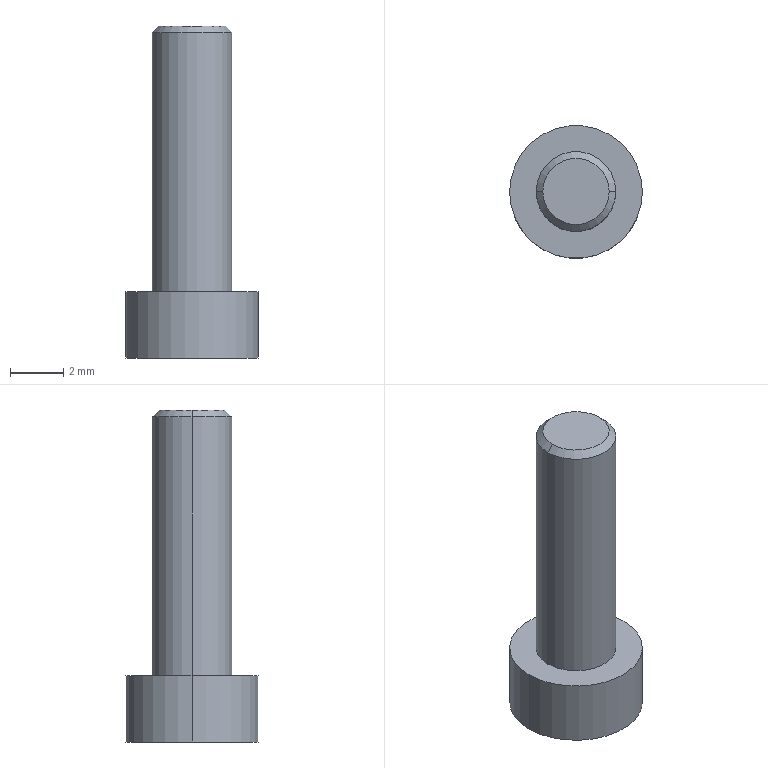Part | SolidWorks | features BaseBody 1 | 1 solid | 16 faces | box 5 x 5 x 12.5 mm | volume 109.752 mm3 | plane 10 | cylinder 4 | cone 2 | commonest cylinder face diameters 3 x2 5 x2
STEP:
#1=CARTESIAN_POINT('',(-1.25,0.,12.5));
#2=VERTEX_POINT('',#1);
#3=CARTESIAN_POINT('',(1.25,0.,12.5));
#4=VERTEX_POINT('',#3);
#5=CARTESIAN_POINT('',(0.,0.,12.5));
#6=DIRECTION('',(0.,0.,-1.));
#7=DIRECTION('',(-1.,0.,0.));
#8=AXIS2_PLACEMENT_3D('',#5,#6,#7);
#9=CIRCLE('',#8,1.25);
#10=EDGE_CURVE('',#2,#4,#9,.T.);
#11=ORIENTED_EDGE('',*,*,#10,.T.);
#12=CARTESIAN_POINT('',(1.5,0.,12.25));
#13=VERTEX_POINT('',#12);
#14=CARTESIAN_POINT('',(1.375,0.,12.375));
#15=DIRECTION('',(0.7071,0.,-0.7071));
#16=VECTOR('',#15,1000.);
#17=LINE('',#14,#16);
#18=EDGE_CURVE('',#4,#13,#17,.T.);
#19=ORIENTED_EDGE('',*,*,#18,.T.);
#20=CARTESIAN_POINT('',(-1.5,0.,12.25));
#21=VERTEX_POINT('',#20);
#22=CARTESIAN_POINT('',(0.,0.,12.25));
#23=DIRECTION('',(0.,0.,1.));
#24=DIRECTION('',(-1.,0.,0.));
#25=AXIS2_PLACEMENT_3D('',#22,#23,#24);
#26=CIRCLE('',#25,1.5);
#27=EDGE_CURVE('',#13,#21,#26,.T.);
#28=ORIENTED_EDGE('',*,*,#27,.T.);
#29=CARTESIAN_POINT('',(-1.375,0.,12.375));
#30=DIRECTION('',(-0.7071,0.,-0.7071));
#31=VECTOR('',#30,1000.);
#32=LINE('',#29,#31);
#33=EDGE_CURVE('',#2,#21,#32,.T.);
#34=ORIENTED_EDGE('',*,*,#33,.F.);
#35=EDGE_LOOP('',(#11,#19,#28,#34));
#36=FACE_OUTER_BOUND('',#35,.T.);
#37=CARTESIAN_POINT('',(0.,0.,12.375));
#38=DIRECTION('',(0.,0.,-1.));
#39=DIRECTION('',(-1.,0.,0.));
#40=AXIS2_PLACEMENT_3D('',#37,#38,#39);
#41=CONICAL_SURFACE('',#40,1.375,0.7854);
#42=ADVANCED_FACE('',(#36),#41,.T.);
#43=ORIENTED_EDGE('',*,*,#27,.F.);
#44=CARTESIAN_POINT('',(1.5,0.,2.5));
#45=VERTEX_POINT('',#44);
#46=CARTESIAN_POINT('',(1.5,0.,2.5));
#47=DIRECTION('',(0.,0.,-1.));
#48=VECTOR('',#47,1000.);
#49=LINE('',#46,#48);
#50=EDGE_CURVE('',#13,#45,#49,.T.);
#51=ORIENTED_EDGE('',*,*,#50,.T.);
#52=CARTESIAN_POINT('',(-1.5,0.,2.5));
#53=VERTEX_POINT('',#52);
#54=CARTESIAN_POINT('',(0.,0.,2.5));
#55=DIRECTION('',(0.,0.,-1.));
#56=DIRECTION('',(-1.,0.,0.));
#57=AXIS2_PLACEMENT_3D('',#54,#55,#56);
#58=CIRCLE('',#57,1.5);
#59=EDGE_CURVE('',#53,#45,#58,.T.);
#60=ORIENTED_EDGE('',*,*,#59,.F.);
#61=CARTESIAN_POINT('',(-1.5,0.,2.5));
#62=DIRECTION('',(0.,0.,-1.));
#63=VECTOR('',#62,1000.);
#64=LINE('',#61,#63);
#65=EDGE_CURVE('',#21,#53,#64,.T.);
#66=ORIENTED_EDGE('',*,*,#65,.F.);
#67=EDGE_LOOP('',(#43,#51,#60,#66));
#68=FACE_OUTER_BOUND('',#67,.T.);
#69=CARTESIAN_POINT('',(0.,0.,2.5));
#70=DIRECTION('',(0.,0.,-1.));
#71=DIRECTION('',(-1.,0.,0.));
#72=AXIS2_PLACEMENT_3D('',#69,#70,#71);
#73=CYLINDRICAL_SURFACE('',#72,1.5);
#74=ADVANCED_FACE('',(#68),#73,.T.);
#75=CARTESIAN_POINT('',(2.5,0.,2.5));
#76=VERTEX_POINT('',#75);
#77=CARTESIAN_POINT('',(-2.5,0.,2.5));
#78=VERTEX_POINT('',#77);
#79=CARTESIAN_POINT('',(0.,0.,2.5));
#80=DIRECTION('',(0.,0.,1.));
#81=DIRECTION('',(-1.,0.,0.));
#82=AXIS2_PLACEMENT_3D('',#79,#80,#81);
#83=CIRCLE('',#82,2.5);
#84=EDGE_CURVE('',#76,#78,#83,.T.);
#85=ORIENTED_EDGE('',*,*,#84,.F.);
#86=CARTESIAN_POINT('',(2.5,0.,0.));
#87=VERTEX_POINT('',#86);
#88=CARTESIAN_POINT('',(2.5,0.,0.));
#89=DIRECTION('',(0.,0.,-1.));
#90=VECTOR('',#89,1000.);
#91=LINE('',#88,#90);
#92=EDGE_CURVE('',#76,#87,#91,.T.);
#93=ORIENTED_EDGE('',*,*,#92,.T.);
#94=CARTESIAN_POINT('',(-2.5,0.,0.));
#95=VERTEX_POINT('',#94);
#96=CARTESIAN_POINT('',(0.,0.,0.));
#97=DIRECTION('',(0.,0.,-1.));
#98=DIRECTION('',(-1.,0.,0.));
#99=AXIS2_PLACEMENT_3D('',#96,#97,#98);
#100=CIRCLE('',#99,2.5);
#101=EDGE_CURVE('',#95,#87,#100,.T.);
#102=ORIENTED_EDGE('',*,*,#101,.F.);
#103=CARTESIAN_POINT('',(-2.5,0.,0.));
#104=DIRECTION('',(0.,0.,-1.));
#105=VECTOR('',#104,1000.);
#106=LINE('',#103,#105);
#107=EDGE_CURVE('',#78,#95,#106,.T.);
#108=ORIENTED_EDGE('',*,*,#107,.F.);
#109=EDGE_LOOP('',(#85,#93,#102,#108));
#110=FACE_OUTER_BOUND('',#109,.T.);
#111=CARTESIAN_POINT('',(0.,0.,0.));
#112=DIRECTION('',(0.,0.,-1.));
#113=DIRECTION('',(-1.,0.,0.));
#114=AXIS2_PLACEMENT_3D('',#111,#112,#113);
#115=CYLINDRICAL_SURFACE('',#114,2.5);
#116=ADVANCED_FACE('',(#110),#115,.T.);
#117=CARTESIAN_POINT('',(-1.732,0.,0.));
#118=VERTEX_POINT('',#117);
#119=CARTESIAN_POINT('',(-0.866,-1.5,0.));
#120=VERTEX_POINT('',#119);
#121=CARTESIAN_POINT('',(-1.516,-0.375,0.));
#122=DIRECTION('',(0.5,-0.866,0.));
#123=VECTOR('',#122,1000.);
#124=LINE('',#121,#123);
#125=EDGE_CURVE('',#118,#120,#124,.T.);
#126=ORIENTED_EDGE('',*,*,#125,.F.);
#127=CARTESIAN_POINT('',(-1.732,0.,1.25));
#128=VERTEX_POINT('',#127);
#129=CARTESIAN_POINT('',(-1.732,0.,0.));
#130=DIRECTION('',(0.,0.,1.));
#131=VECTOR('',#130,1000.);
#132=LINE('',#129,#131);
#133=EDGE_CURVE('',#118,#128,#132,.T.);
#134=ORIENTED_EDGE('',*,*,#133,.T.);
#135=CARTESIAN_POINT('',(-0.866,-1.5,1.25));
#136=VERTEX_POINT('',#135);
#137=CARTESIAN_POINT('',(-1.732,0.,1.25));
#138=DIRECTION('',(0.5,-0.866,0.));
#139=VECTOR('',#138,1000.);
#140=LINE('',#137,#139);
#141=EDGE_CURVE('',#128,#136,#140,.T.);
#142=ORIENTED_EDGE('',*,*,#141,.T.);
#143=CARTESIAN_POINT('',(-0.866,-1.5,0.));
#144=DIRECTION('',(0.,0.,1.));
#145=VECTOR('',#144,1000.);
#146=LINE('',#143,#145);
#147=EDGE_CURVE('',#120,#136,#146,.T.);
#148=ORIENTED_EDGE('',*,*,#147,.F.);
#149=EDGE_LOOP('',(#126,#134,#142,#148));
#150=FACE_OUTER_BOUND('',#149,.T.);
#151=CARTESIAN_POINT('',(-1.732,0.,0.));
#152=DIRECTION('',(-0.866,-0.5,0.));
#153=DIRECTION('',(-0.5,0.866,0.));
#154=AXIS2_PLACEMENT_3D('',#151,#152,#153);
#155=PLANE('',#154);
#156=ADVANCED_FACE('',(#150),#155,.F.);
#157=CARTESIAN_POINT('',(-0.866,1.5,0.));
#158=VERTEX_POINT('',#157);
#159=CARTESIAN_POINT('',(-1.083,1.125,0.));
#160=DIRECTION('',(-0.5,-0.866,0.));
#161=VECTOR('',#160,1000.);
#162=LINE('',#159,#161);
#163=EDGE_CURVE('',#158,#118,#162,.T.);
#164=ORIENTED_EDGE('',*,*,#163,.F.);
#165=CARTESIAN_POINT('',(-0.866,1.5,1.25));
#166=VERTEX_POINT('',#165);
#167=CARTESIAN_POINT('',(-0.866,1.5,0.));
#168=DIRECTION('',(0.,0.,1.));
#169=VECTOR('',#168,1000.);
#170=LINE('',#167,#169);
#171=EDGE_CURVE('',#158,#166,#170,.T.);
#172=ORIENTED_EDGE('',*,*,#171,.T.);
#173=CARTESIAN_POINT('',(-0.866,1.5,1.25));
#174=DIRECTION('',(-0.5,-0.866,0.));
#175=VECTOR('',#174,1000.);
#176=LINE('',#173,#175);
#177=EDGE_CURVE('',#166,#128,#176,.T.);
#178=ORIENTED_EDGE('',*,*,#177,.T.);
#179=ORIENTED_EDGE('',*,*,#133,.F.);
#180=EDGE_LOOP('',(#164,#172,#178,#179));
#181=FACE_OUTER_BOUND('',#180,.T.);
#182=CARTESIAN_POINT('',(-0.866,1.5,0.));
#183=DIRECTION('',(-0.866,0.5,0.));
#184=DIRECTION('',(0.,0.,1.));
#185=AXIS2_PLACEMENT_3D('',#182,#183,#184);
#186=PLANE('',#185);
#187=ADVANCED_FACE('',(#181),#186,.F.);
#188=CARTESIAN_POINT('',(0.866,1.5,0.));
#189=VERTEX_POINT('',#188);
#190=CARTESIAN_POINT('',(0.433,1.5,0.));
#191=DIRECTION('',(-1.,0.,0.));
#192=VECTOR('',#191,1000.);
#193=LINE('',#190,#192);
#194=EDGE_CURVE('',#189,#158,#193,.T.);
#195=ORIENTED_EDGE('',*,*,#194,.F.);
#196=CARTESIAN_POINT('',(0.866,1.5,1.25));
#197=VERTEX_POINT('',#196);
#198=CARTESIAN_POINT('',(0.866,1.5,0.));
#199=DIRECTION('',(0.,0.,1.));
#200=VECTOR('',#199,1000.);
#201=LINE('',#198,#200);
#202=EDGE_CURVE('',#189,#197,#201,.T.);
#203=ORIENTED_EDGE('',*,*,#202,.T.);
#204=CARTESIAN_POINT('',(0.866,1.5,1.25));
#205=DIRECTION('',(-1.,0.,0.));
#206=VECTOR('',#205,1000.);
#207=LINE('',#204,#206);
#208=EDGE_CURVE('',#197,#166,#207,.T.);
#209=ORIENTED_EDGE('',*,*,#208,.T.);
#210=ORIENTED_EDGE('',*,*,#171,.F.);
#211=EDGE_LOOP('',(#195,#203,#209,#210));
#212=FACE_OUTER_BOUND('',#211,.T.);
#213=CARTESIAN_POINT('',(0.866,1.5,0.));
#214=DIRECTION('',(0.,1.,0.));
#215=DIRECTION('',(1.,0.,0.));
#216=AXIS2_PLACEMENT_3D('',#213,#214,#215);
#217=PLANE('',#216);
#218=ADVANCED_FACE('',(#212),#217,.F.);
#219=CARTESIAN_POINT('',(1.732,0.,0.));
#220=VERTEX_POINT('',#219);
#221=CARTESIAN_POINT('',(1.516,0.375,0.));
#222=DIRECTION('',(-0.5,0.866,0.));
#223=VECTOR('',#222,1000.);
#224=LINE('',#221,#223);
#225=EDGE_CURVE('',#220,#189,#224,.T.);
#226=ORIENTED_EDGE('',*,*,#225,.F.);
#227=CARTESIAN_POINT('',(1.732,0.,1.25));
#228=VERTEX_POINT('',#227);
#229=CARTESIAN_POINT('',(1.732,0.,0.));
#230=DIRECTION('',(0.,0.,1.));
#231=VECTOR('',#230,1000.);
#232=LINE('',#229,#231);
#233=EDGE_CURVE('',#220,#228,#232,.T.);
#234=ORIENTED_EDGE('',*,*,#233,.T.);
#235=CARTESIAN_POINT('',(1.732,0.,1.25));
#236=DIRECTION('',(-0.5,0.866,0.));
#237=VECTOR('',#236,1000.);
#238=LINE('',#235,#237);
#239=EDGE_CURVE('',#228,#197,#238,.T.);
#240=ORIENTED_EDGE('',*,*,#239,.T.);
#241=ORIENTED_EDGE('',*,*,#202,.F.);
#242=EDGE_LOOP('',(#226,#234,#240,#241));
#243=FACE_OUTER_BOUND('',#242,.T.);
#244=CARTESIAN_POINT('',(1.732,0.,0.));
#245=DIRECTION('',(0.866,0.5,0.));
#246=DIRECTION('',(0.,0.,-1.));
#247=AXIS2_PLACEMENT_3D('',#244,#245,#246);
#248=PLANE('',#247);
#249=ADVANCED_FACE('',(#243),#248,.F.);
#250=CARTESIAN_POINT('',(0.866,-1.5,0.));
#251=VERTEX_POINT('',#250);
#252=CARTESIAN_POINT('',(1.083,-1.125,0.));
#253=DIRECTION('',(0.5,0.866,0.));
#254=VECTOR('',#253,1000.);
#255=LINE('',#252,#254);
#256=EDGE_CURVE('',#251,#220,#255,.T.);
#257=ORIENTED_EDGE('',*,*,#256,.F.);
#258=CARTESIAN_POINT('',(0.866,-1.5,1.25));
#259=VERTEX_POINT('',#258);
#260=CARTESIAN_POINT('',(0.866,-1.5,0.));
#261=DIRECTION('',(0.,0.,1.));
#262=VECTOR('',#261,1000.);
#263=LINE('',#260,#262);
#264=EDGE_CURVE('',#251,#259,#263,.T.);
#265=ORIENTED_EDGE('',*,*,#264,.T.);
#266=CARTESIAN_POINT('',(0.866,-1.5,1.25));
#267=DIRECTION('',(0.5,0.866,0.));
#268=VECTOR('',#267,1000.);
#269=LINE('',#266,#268);
#270=EDGE_CURVE('',#259,#228,#269,.T.);
#271=ORIENTED_EDGE('',*,*,#270,.T.);
#272=ORIENTED_EDGE('',*,*,#233,.F.);
#273=EDGE_LOOP('',(#257,#265,#271,#272));
#274=FACE_OUTER_BOUND('',#273,.T.);
#275=CARTESIAN_POINT('',(0.866,-1.5,0.));
#276=DIRECTION('',(0.866,-0.5,0.));
#277=DIRECTION('',(0.,0.,-1.));
#278=AXIS2_PLACEMENT_3D('',#275,#276,#277);
#279=PLANE('',#278);
#280=ADVANCED_FACE('',(#274),#279,.F.);
#281=CARTESIAN_POINT('',(-0.433,-1.5,0.));
#282=DIRECTION('',(1.,0.,0.));
#283=VECTOR('',#282,1000.);
#284=LINE('',#281,#283);
#285=EDGE_CURVE('',#120,#251,#284,.T.);
#286=ORIENTED_EDGE('',*,*,#285,.F.);
#287=ORIENTED_EDGE('',*,*,#147,.T.);
#288=CARTESIAN_POINT('',(-0.866,-1.5,1.25));
#289=DIRECTION('',(1.,0.,0.));
#290=VECTOR('',#289,1000.);
#291=LINE('',#288,#290);
#292=EDGE_CURVE('',#136,#259,#291,.T.);
#293=ORIENTED_EDGE('',*,*,#292,.T.);
#294=ORIENTED_EDGE('',*,*,#264,.F.);
#295=EDGE_LOOP('',(#286,#287,#293,#294));
#296=FACE_OUTER_BOUND('',#295,.T.);
#297=CARTESIAN_POINT('',(-0.866,-1.5,0.));
#298=DIRECTION('',(0.,-1.,0.));
#299=DIRECTION('',(0.,0.,-1.));
#300=AXIS2_PLACEMENT_3D('',#297,#298,#299);
#301=PLANE('',#300);
#302=ADVANCED_FACE('',(#296),#301,.F.);
#303=ORIENTED_EDGE('',*,*,#292,.F.);
#304=ORIENTED_EDGE('',*,*,#141,.F.);
#305=ORIENTED_EDGE('',*,*,#177,.F.);
#306=ORIENTED_EDGE('',*,*,#208,.F.);
#307=ORIENTED_EDGE('',*,*,#239,.F.);
#308=ORIENTED_EDGE('',*,*,#270,.F.);
#309=EDGE_LOOP('',(#303,#304,#305,#306,#307,#308));
#310=FACE_OUTER_BOUND('',#309,.T.);
#311=CARTESIAN_POINT('',(0.,0.,1.25));
#312=DIRECTION('',(0.,0.,1.));
#313=DIRECTION('',(1.,0.,0.));
#314=AXIS2_PLACEMENT_3D('',#311,#312,#313);
#315=PLANE('',#314);
#316=ADVANCED_FACE('',(#310),#315,.F.);
#317=ORIENTED_EDGE('',*,*,#10,.F.);
#318=CARTESIAN_POINT('',(0.,0.,12.5));
#319=DIRECTION('',(0.,0.,-1.));
#320=DIRECTION('',(-1.,0.,0.));
#321=AXIS2_PLACEMENT_3D('',#318,#319,#320);
#322=CIRCLE('',#321,1.25);
#323=EDGE_CURVE('',#4,#2,#322,.T.);
#324=ORIENTED_EDGE('',*,*,#323,.F.);
#325=EDGE_LOOP('',(#317,#324));
#326=FACE_OUTER_BOUND('',#325,.T.);
#327=CARTESIAN_POINT('',(0.,0.,12.5));
#328=DIRECTION('',(0.,0.,1.));
#329=DIRECTION('',(1.,0.,0.));
#330=AXIS2_PLACEMENT_3D('',#327,#328,#329);
#331=PLANE('',#330);
#332=ADVANCED_FACE('',(#326),#331,.T.);
#333=ORIENTED_EDGE('',*,*,#125,.T.);
#334=ORIENTED_EDGE('',*,*,#285,.T.);
#335=ORIENTED_EDGE('',*,*,#256,.T.);
#336=ORIENTED_EDGE('',*,*,#225,.T.);
#337=ORIENTED_EDGE('',*,*,#194,.T.);
#338=ORIENTED_EDGE('',*,*,#163,.T.);
#339=EDGE_LOOP('',(#333,#334,#335,#336,#337,#338));
#340=FACE_BOUND('',#339,.T.);
#341=ORIENTED_EDGE('',*,*,#101,.T.);
#342=CARTESIAN_POINT('',(0.,0.,0.));
#343=DIRECTION('',(0.,0.,-1.));
#344=DIRECTION('',(-1.,0.,0.));
#345=AXIS2_PLACEMENT_3D('',#342,#343,#344);
#346=CIRCLE('',#345,2.5);
#347=EDGE_CURVE('',#87,#95,#346,.T.);
#348=ORIENTED_EDGE('',*,*,#347,.T.);
#349=EDGE_LOOP('',(#341,#348));
#350=FACE_OUTER_BOUND('',#349,.T.);
#351=CARTESIAN_POINT('',(0.,0.,0.));
#352=DIRECTION('',(0.,0.,1.));
#353=DIRECTION('',(1.,0.,0.));
#354=AXIS2_PLACEMENT_3D('',#351,#352,#353);
#355=PLANE('',#354);
#356=ADVANCED_FACE('',(#340,#350),#355,.F.);
#357=ORIENTED_EDGE('',*,*,#59,.T.);
#358=CARTESIAN_POINT('',(0.,0.,2.5));
#359=DIRECTION('',(0.,0.,-1.));
#360=DIRECTION('',(-1.,0.,0.));
#361=AXIS2_PLACEMENT_3D('',#358,#359,#360);
#362=CIRCLE('',#361,1.5);
#363=EDGE_CURVE('',#45,#53,#362,.T.);
#364=ORIENTED_EDGE('',*,*,#363,.T.);
#365=EDGE_LOOP('',(#357,#364));
#366=FACE_BOUND('',#365,.T.);
#367=CARTESIAN_POINT('',(0.,0.,2.5));
#368=DIRECTION('',(0.,0.,1.));
#369=DIRECTION('',(-1.,0.,0.));
#370=AXIS2_PLACEMENT_3D('',#367,#368,#369);
#371=CIRCLE('',#370,2.5);
#372=EDGE_CURVE('',#78,#76,#371,.T.);
#373=ORIENTED_EDGE('',*,*,#372,.T.);
#374=ORIENTED_EDGE('',*,*,#84,.T.);
#375=EDGE_LOOP('',(#373,#374));
#376=FACE_OUTER_BOUND('',#375,.T.);
#377=CARTESIAN_POINT('',(0.,0.,2.5));
#378=DIRECTION('',(0.,0.,1.));
#379=DIRECTION('',(1.,0.,0.));
#380=AXIS2_PLACEMENT_3D('',#377,#378,#379);
#381=PLANE('',#380);
#382=ADVANCED_FACE('',(#366,#376),#381,.T.);
#383=ORIENTED_EDGE('',*,*,#92,.F.);
#384=ORIENTED_EDGE('',*,*,#372,.F.);
#385=ORIENTED_EDGE('',*,*,#107,.T.);
#386=ORIENTED_EDGE('',*,*,#347,.F.);
#387=EDGE_LOOP('',(#383,#384,#385,#386));
#388=FACE_OUTER_BOUND('',#387,.T.);
#389=CARTESIAN_POINT('',(0.,0.,0.));
#390=DIRECTION('',(0.,0.,-1.));
#391=DIRECTION('',(-1.,0.,0.));
#392=AXIS2_PLACEMENT_3D('',#389,#390,#391);
#393=CYLINDRICAL_SURFACE('',#392,2.5);
#394=ADVANCED_FACE('',(#388),#393,.T.);
#395=ORIENTED_EDGE('',*,*,#50,.F.);
#396=CARTESIAN_POINT('',(0.,0.,12.25));
#397=DIRECTION('',(0.,0.,1.));
#398=DIRECTION('',(-1.,0.,0.));
#399=AXIS2_PLACEMENT_3D('',#396,#397,#398);
#400=CIRCLE('',#399,1.5);
#401=EDGE_CURVE('',#21,#13,#400,.T.);
#402=ORIENTED_EDGE('',*,*,#401,.F.);
#403=ORIENTED_EDGE('',*,*,#65,.T.);
#404=ORIENTED_EDGE('',*,*,#363,.F.);
#405=EDGE_LOOP('',(#395,#402,#403,#404));
#406=FACE_OUTER_BOUND('',#405,.T.);
#407=CARTESIAN_POINT('',(0.,0.,2.5));
#408=DIRECTION('',(0.,0.,-1.));
#409=DIRECTION('',(-1.,0.,0.));
#410=AXIS2_PLACEMENT_3D('',#407,#408,#409);
#411=CYLINDRICAL_SURFACE('',#410,1.5);
#412=ADVANCED_FACE('',(#406),#411,.T.);
#413=ORIENTED_EDGE('',*,*,#18,.F.);
#414=ORIENTED_EDGE('',*,*,#323,.T.);
#415=ORIENTED_EDGE('',*,*,#33,.T.);
#416=ORIENTED_EDGE('',*,*,#401,.T.);
#417=EDGE_LOOP('',(#413,#414,#415,#416));
#418=FACE_OUTER_BOUND('',#417,.T.);
#419=CARTESIAN_POINT('',(0.,0.,12.375));
#420=DIRECTION('',(0.,0.,-1.));
#421=DIRECTION('',(-1.,0.,0.));
#422=AXIS2_PLACEMENT_3D('',#419,#420,#421);
#423=CONICAL_SURFACE('',#422,1.375,0.7854);
#424=ADVANCED_FACE('',(#418),#423,.T.);
#425=CLOSED_SHELL('',(#42,#74,#116,#156,#187,#218,#249,#280,#302,#316,#332,#356,#382,#394,#412,#424));
#426=MANIFOLD_SOLID_BREP('',#425);
#427=CARTESIAN_POINT('',(0.,0.,0.));
#428=DIRECTION('',(0.,0.,1.));
#429=DIRECTION('',(1.,0.,0.));
#430=AXIS2_PLACEMENT_3D('',#427,#428,#429);
#431=(LENGTH_UNIT()NAMED_UNIT(*)SI_UNIT(.MILLI.,.METRE.));
#432=UNCERTAINTY_MEASURE_WITH_UNIT(LENGTH_MEASURE(0.00001),#431,'','');
#433=(NAMED_UNIT(*)PLANE_ANGLE_UNIT()SI_UNIT($,.RADIAN.));
#434=(NAMED_UNIT(*)SI_UNIT($,.STERADIAN.)SOLID_ANGLE_UNIT());
#435=(GEOMETRIC_REPRESENTATION_CONTEXT(3)GLOBAL_UNCERTAINTY_ASSIGNED_CONTEXT((#432))GLOBAL_UNIT_ASSIGNED_CONTEXT((#431,#433,#434))REPRESENTATION_CONTEXT('',''));
#436=ADVANCED_BREP_SHAPE_REPRESENTATION('',(#426,#430),#435);